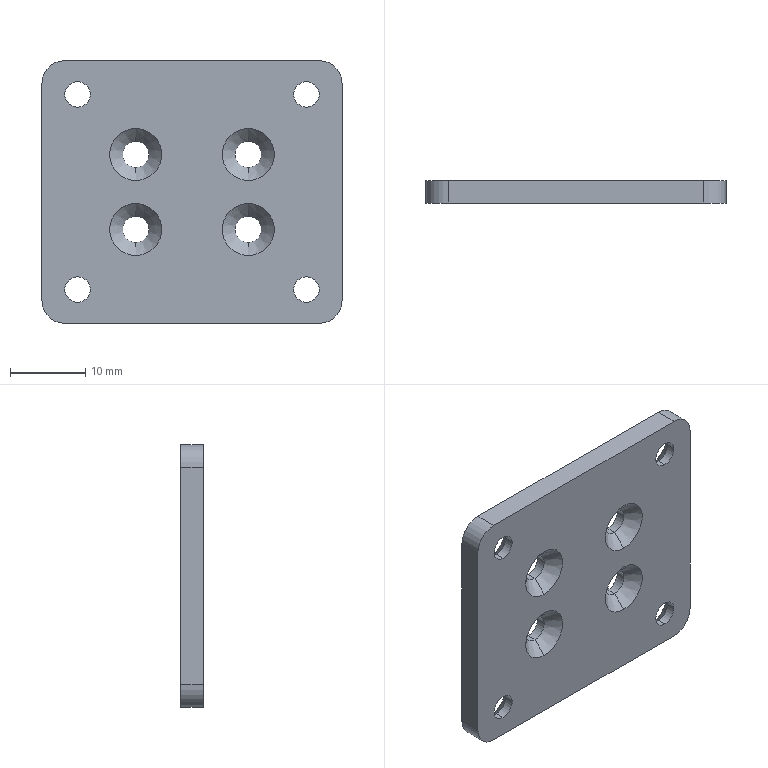Part | STEP file | MGN9C slider mounting base plate 1001 | 1 solid | 42 faces | box 40 x 3 x 35 mm | volume 3776 mm3 | cylinder 20 | cone 16 | plane 6 | commonest cylinder face diameters 3.4 x8 3.5 x8 6 x4